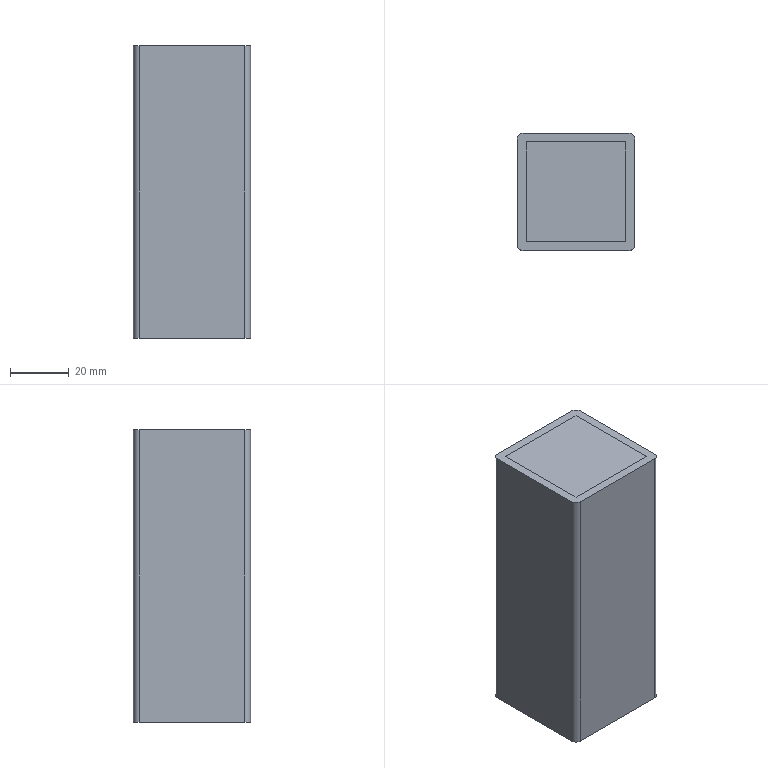Part | STEP file | X77-09105 | 2 solids | 20 faces | box 40 x 40 x 100 mm | volume 48681 mm3 | plane 16 | cylinder 4 | commonest cylinder face diameters 4 x4
STEP:
#1=CARTESIAN_POINT('',(0.,2.,100.));
#2=VERTEX_POINT('',#1);
#3=CARTESIAN_POINT('',(2.,0.,100.));
#4=VERTEX_POINT('',#3);
#5=CARTESIAN_POINT('',(2.,2.,100.));
#6=DIRECTION('',(0.,0.,1.));
#7=DIRECTION('',(1.,0.,0.));
#8=AXIS2_PLACEMENT_3D('',#5,#6,#7);
#9=CIRCLE('',#8,2.);
#10=EDGE_CURVE('',#2,#4,#9,.T.);
#11=ORIENTED_EDGE('',*,*,#10,.T.);
#12=CARTESIAN_POINT('',(38.,0.,100.));
#13=VERTEX_POINT('',#12);
#14=CARTESIAN_POINT('',(2.,0.,100.));
#15=DIRECTION('',(1.,0.,0.));
#16=VECTOR('',#15,1000.);
#17=LINE('',#14,#16);
#18=EDGE_CURVE('',#4,#13,#17,.T.);
#19=ORIENTED_EDGE('',*,*,#18,.T.);
#20=CARTESIAN_POINT('',(40.,2.,100.));
#21=VERTEX_POINT('',#20);
#22=CARTESIAN_POINT('',(38.,2.,100.));
#23=DIRECTION('',(0.,0.,1.));
#24=DIRECTION('',(1.,0.,0.));
#25=AXIS2_PLACEMENT_3D('',#22,#23,#24);
#26=CIRCLE('',#25,2.);
#27=EDGE_CURVE('',#13,#21,#26,.T.);
#28=ORIENTED_EDGE('',*,*,#27,.T.);
#29=CARTESIAN_POINT('',(40.,38.,100.));
#30=VERTEX_POINT('',#29);
#31=CARTESIAN_POINT('',(40.,2.,100.));
#32=DIRECTION('',(0.,1.,0.));
#33=VECTOR('',#32,1000.);
#34=LINE('',#31,#33);
#35=EDGE_CURVE('',#21,#30,#34,.T.);
#36=ORIENTED_EDGE('',*,*,#35,.T.);
#37=CARTESIAN_POINT('',(38.,40.,100.));
#38=VERTEX_POINT('',#37);
#39=CARTESIAN_POINT('',(38.,38.,100.));
#40=DIRECTION('',(0.,0.,1.));
#41=DIRECTION('',(1.,0.,0.));
#42=AXIS2_PLACEMENT_3D('',#39,#40,#41);
#43=CIRCLE('',#42,2.);
#44=EDGE_CURVE('',#30,#38,#43,.T.);
#45=ORIENTED_EDGE('',*,*,#44,.T.);
#46=CARTESIAN_POINT('',(2.,40.,100.));
#47=VERTEX_POINT('',#46);
#48=CARTESIAN_POINT('',(2.,40.,100.));
#49=DIRECTION('',(-1.,0.,0.));
#50=VECTOR('',#49,1000.);
#51=LINE('',#48,#50);
#52=EDGE_CURVE('',#38,#47,#51,.T.);
#53=ORIENTED_EDGE('',*,*,#52,.T.);
#54=CARTESIAN_POINT('',(0.,38.,100.));
#55=VERTEX_POINT('',#54);
#56=CARTESIAN_POINT('',(2.,38.,100.));
#57=DIRECTION('',(0.,0.,1.));
#58=DIRECTION('',(-1.,0.,0.));
#59=AXIS2_PLACEMENT_3D('',#56,#57,#58);
#60=CIRCLE('',#59,2.);
#61=EDGE_CURVE('',#47,#55,#60,.T.);
#62=ORIENTED_EDGE('',*,*,#61,.T.);
#63=CARTESIAN_POINT('',(0.,2.,100.));
#64=DIRECTION('',(0.,-1.,0.));
#65=VECTOR('',#64,1000.);
#66=LINE('',#63,#65);
#67=EDGE_CURVE('',#55,#2,#66,.T.);
#68=ORIENTED_EDGE('',*,*,#67,.T.);
#69=EDGE_LOOP('',(#11,#19,#28,#36,#45,#53,#62,#68));
#70=FACE_OUTER_BOUND('',#69,.T.);
#71=CARTESIAN_POINT('',(3.,3.,100.));
#72=VERTEX_POINT('',#71);
#73=CARTESIAN_POINT('',(37.,3.,100.));
#74=VERTEX_POINT('',#73);
#75=CARTESIAN_POINT('',(3.,3.,100.));
#76=DIRECTION('',(1.,0.,0.));
#77=VECTOR('',#76,1000.);
#78=LINE('',#75,#77);
#79=EDGE_CURVE('',#72,#74,#78,.T.);
#80=ORIENTED_EDGE('',*,*,#79,.F.);
#81=CARTESIAN_POINT('',(3.,37.,100.));
#82=VERTEX_POINT('',#81);
#83=CARTESIAN_POINT('',(3.,3.,100.));
#84=DIRECTION('',(0.,-1.,0.));
#85=VECTOR('',#84,1000.);
#86=LINE('',#83,#85);
#87=EDGE_CURVE('',#82,#72,#86,.T.);
#88=ORIENTED_EDGE('',*,*,#87,.F.);
#89=CARTESIAN_POINT('',(37.,37.,100.));
#90=VERTEX_POINT('',#89);
#91=CARTESIAN_POINT('',(3.,37.,100.));
#92=DIRECTION('',(-1.,0.,0.));
#93=VECTOR('',#92,1000.);
#94=LINE('',#91,#93);
#95=EDGE_CURVE('',#90,#82,#94,.T.);
#96=ORIENTED_EDGE('',*,*,#95,.F.);
#97=CARTESIAN_POINT('',(37.,3.,100.));
#98=DIRECTION('',(0.,1.,0.));
#99=VECTOR('',#98,1000.);
#100=LINE('',#97,#99);
#101=EDGE_CURVE('',#74,#90,#100,.T.);
#102=ORIENTED_EDGE('',*,*,#101,.F.);
#103=EDGE_LOOP('',(#80,#88,#96,#102));
#104=FACE_BOUND('',#103,.T.);
#105=CARTESIAN_POINT('',(2.,2.,100.));
#106=DIRECTION('',(0.,0.,1.));
#107=DIRECTION('',(1.,0.,0.));
#108=AXIS2_PLACEMENT_3D('',#105,#106,#107);
#109=PLANE('',#108);
#110=ADVANCED_FACE('',(#70,#104),#109,.T.);
#111=CARTESIAN_POINT('',(0.,2.,0.));
#112=VERTEX_POINT('',#111);
#113=CARTESIAN_POINT('',(2.,0.,0.));
#114=VERTEX_POINT('',#113);
#115=CARTESIAN_POINT('',(2.,2.,0.));
#116=DIRECTION('',(0.,0.,1.));
#117=DIRECTION('',(1.,0.,0.));
#118=AXIS2_PLACEMENT_3D('',#115,#116,#117);
#119=CIRCLE('',#118,2.);
#120=EDGE_CURVE('',#112,#114,#119,.T.);
#121=ORIENTED_EDGE('',*,*,#120,.F.);
#122=CARTESIAN_POINT('',(0.,38.,0.));
#123=VERTEX_POINT('',#122);
#124=CARTESIAN_POINT('',(0.,2.,0.));
#125=DIRECTION('',(0.,-1.,0.));
#126=VECTOR('',#125,1000.);
#127=LINE('',#124,#126);
#128=EDGE_CURVE('',#123,#112,#127,.T.);
#129=ORIENTED_EDGE('',*,*,#128,.F.);
#130=CARTESIAN_POINT('',(2.,40.,0.));
#131=VERTEX_POINT('',#130);
#132=CARTESIAN_POINT('',(2.,38.,0.));
#133=DIRECTION('',(0.,0.,1.));
#134=DIRECTION('',(-1.,0.,0.));
#135=AXIS2_PLACEMENT_3D('',#132,#133,#134);
#136=CIRCLE('',#135,2.);
#137=EDGE_CURVE('',#131,#123,#136,.T.);
#138=ORIENTED_EDGE('',*,*,#137,.F.);
#139=CARTESIAN_POINT('',(38.,40.,0.));
#140=VERTEX_POINT('',#139);
#141=CARTESIAN_POINT('',(2.,40.,0.));
#142=DIRECTION('',(-1.,0.,0.));
#143=VECTOR('',#142,1000.);
#144=LINE('',#141,#143);
#145=EDGE_CURVE('',#140,#131,#144,.T.);
#146=ORIENTED_EDGE('',*,*,#145,.F.);
#147=CARTESIAN_POINT('',(40.,38.,0.));
#148=VERTEX_POINT('',#147);
#149=CARTESIAN_POINT('',(38.,38.,0.));
#150=DIRECTION('',(0.,0.,1.));
#151=DIRECTION('',(1.,0.,0.));
#152=AXIS2_PLACEMENT_3D('',#149,#150,#151);
#153=CIRCLE('',#152,2.);
#154=EDGE_CURVE('',#148,#140,#153,.T.);
#155=ORIENTED_EDGE('',*,*,#154,.F.);
#156=CARTESIAN_POINT('',(40.,2.,0.));
#157=VERTEX_POINT('',#156);
#158=CARTESIAN_POINT('',(40.,2.,0.));
#159=DIRECTION('',(0.,1.,0.));
#160=VECTOR('',#159,1000.);
#161=LINE('',#158,#160);
#162=EDGE_CURVE('',#157,#148,#161,.T.);
#163=ORIENTED_EDGE('',*,*,#162,.F.);
#164=CARTESIAN_POINT('',(38.,0.,0.));
#165=VERTEX_POINT('',#164);
#166=CARTESIAN_POINT('',(38.,2.,0.));
#167=DIRECTION('',(0.,0.,1.));
#168=DIRECTION('',(1.,0.,0.));
#169=AXIS2_PLACEMENT_3D('',#166,#167,#168);
#170=CIRCLE('',#169,2.);
#171=EDGE_CURVE('',#165,#157,#170,.T.);
#172=ORIENTED_EDGE('',*,*,#171,.F.);
#173=CARTESIAN_POINT('',(2.,0.,0.));
#174=DIRECTION('',(1.,0.,0.));
#175=VECTOR('',#174,1000.);
#176=LINE('',#173,#175);
#177=EDGE_CURVE('',#114,#165,#176,.T.);
#178=ORIENTED_EDGE('',*,*,#177,.F.);
#179=EDGE_LOOP('',(#121,#129,#138,#146,#155,#163,#172,#178));
#180=FACE_OUTER_BOUND('',#179,.T.);
#181=CARTESIAN_POINT('',(3.,37.,0.));
#182=VERTEX_POINT('',#181);
#183=CARTESIAN_POINT('',(3.,3.,0.));
#184=VERTEX_POINT('',#183);
#185=CARTESIAN_POINT('',(3.,3.,0.));
#186=DIRECTION('',(0.,-1.,0.));
#187=VECTOR('',#186,1000.);
#188=LINE('',#185,#187);
#189=EDGE_CURVE('',#182,#184,#188,.T.);
#190=ORIENTED_EDGE('',*,*,#189,.T.);
#191=CARTESIAN_POINT('',(37.,3.,0.));
#192=VERTEX_POINT('',#191);
#193=CARTESIAN_POINT('',(3.,3.,0.));
#194=DIRECTION('',(1.,0.,0.));
#195=VECTOR('',#194,1000.);
#196=LINE('',#193,#195);
#197=EDGE_CURVE('',#184,#192,#196,.T.);
#198=ORIENTED_EDGE('',*,*,#197,.T.);
#199=CARTESIAN_POINT('',(37.,37.,0.));
#200=VERTEX_POINT('',#199);
#201=CARTESIAN_POINT('',(37.,3.,0.));
#202=DIRECTION('',(0.,1.,0.));
#203=VECTOR('',#202,1000.);
#204=LINE('',#201,#203);
#205=EDGE_CURVE('',#192,#200,#204,.T.);
#206=ORIENTED_EDGE('',*,*,#205,.T.);
#207=CARTESIAN_POINT('',(3.,37.,0.));
#208=DIRECTION('',(-1.,0.,0.));
#209=VECTOR('',#208,1000.);
#210=LINE('',#207,#209);
#211=EDGE_CURVE('',#200,#182,#210,.T.);
#212=ORIENTED_EDGE('',*,*,#211,.T.);
#213=EDGE_LOOP('',(#190,#198,#206,#212));
#214=FACE_BOUND('',#213,.T.);
#215=CARTESIAN_POINT('',(2.,2.,0.));
#216=DIRECTION('',(0.,0.,1.));
#217=DIRECTION('',(1.,0.,0.));
#218=AXIS2_PLACEMENT_3D('',#215,#216,#217);
#219=PLANE('',#218);
#220=ADVANCED_FACE('',(#180,#214),#219,.F.);
#221=ORIENTED_EDGE('',*,*,#120,.T.);
#222=CARTESIAN_POINT('',(2.,0.,100.));
#223=DIRECTION('',(0.,0.,-1.));
#224=VECTOR('',#223,1000.);
#225=LINE('',#222,#224);
#226=EDGE_CURVE('',#4,#114,#225,.T.);
#227=ORIENTED_EDGE('',*,*,#226,.F.);
#228=ORIENTED_EDGE('',*,*,#10,.F.);
#229=CARTESIAN_POINT('',(0.,2.,100.));
#230=DIRECTION('',(0.,0.,-1.));
#231=VECTOR('',#230,1000.);
#232=LINE('',#229,#231);
#233=EDGE_CURVE('',#2,#112,#232,.T.);
#234=ORIENTED_EDGE('',*,*,#233,.T.);
#235=EDGE_LOOP('',(#221,#227,#228,#234));
#236=FACE_OUTER_BOUND('',#235,.T.);
#237=CARTESIAN_POINT('',(2.,2.,100.));
#238=DIRECTION('',(0.,0.,-1.));
#239=DIRECTION('',(-1.,0.,0.));
#240=AXIS2_PLACEMENT_3D('',#237,#238,#239);
#241=CYLINDRICAL_SURFACE('',#240,2.);
#242=ADVANCED_FACE('',(#236),#241,.T.);
#243=ORIENTED_EDGE('',*,*,#177,.T.);
#244=CARTESIAN_POINT('',(38.,0.,100.));
#245=DIRECTION('',(0.,0.,-1.));
#246=VECTOR('',#245,1000.);
#247=LINE('',#244,#246);
#248=EDGE_CURVE('',#13,#165,#247,.T.);
#249=ORIENTED_EDGE('',*,*,#248,.F.);
#250=ORIENTED_EDGE('',*,*,#18,.F.);
#251=ORIENTED_EDGE('',*,*,#226,.T.);
#252=EDGE_LOOP('',(#243,#249,#250,#251));
#253=FACE_OUTER_BOUND('',#252,.T.);
#254=CARTESIAN_POINT('',(2.,0.,100.));
#255=DIRECTION('',(0.,1.,0.));
#256=DIRECTION('',(0.,0.,1.));
#257=AXIS2_PLACEMENT_3D('',#254,#255,#256);
#258=PLANE('',#257);
#259=ADVANCED_FACE('',(#253),#258,.F.);
#260=ORIENTED_EDGE('',*,*,#171,.T.);
#261=CARTESIAN_POINT('',(40.,2.,100.));
#262=DIRECTION('',(0.,0.,-1.));
#263=VECTOR('',#262,1000.);
#264=LINE('',#261,#263);
#265=EDGE_CURVE('',#21,#157,#264,.T.);
#266=ORIENTED_EDGE('',*,*,#265,.F.);
#267=ORIENTED_EDGE('',*,*,#27,.F.);
#268=ORIENTED_EDGE('',*,*,#248,.T.);
#269=EDGE_LOOP('',(#260,#266,#267,#268));
#270=FACE_OUTER_BOUND('',#269,.T.);
#271=CARTESIAN_POINT('',(38.,2.,100.));
#272=DIRECTION('',(0.,0.,-1.));
#273=DIRECTION('',(-1.,0.,0.));
#274=AXIS2_PLACEMENT_3D('',#271,#272,#273);
#275=CYLINDRICAL_SURFACE('',#274,2.);
#276=ADVANCED_FACE('',(#270),#275,.T.);
#277=ORIENTED_EDGE('',*,*,#162,.T.);
#278=CARTESIAN_POINT('',(40.,38.,100.));
#279=DIRECTION('',(0.,0.,-1.));
#280=VECTOR('',#279,1000.);
#281=LINE('',#278,#280);
#282=EDGE_CURVE('',#30,#148,#281,.T.);
#283=ORIENTED_EDGE('',*,*,#282,.F.);
#284=ORIENTED_EDGE('',*,*,#35,.F.);
#285=ORIENTED_EDGE('',*,*,#265,.T.);
#286=EDGE_LOOP('',(#277,#283,#284,#285));
#287=FACE_OUTER_BOUND('',#286,.T.);
#288=CARTESIAN_POINT('',(40.,2.,100.));
#289=DIRECTION('',(-1.,0.,0.));
#290=DIRECTION('',(0.,-1.,0.));
#291=AXIS2_PLACEMENT_3D('',#288,#289,#290);
#292=PLANE('',#291);
#293=ADVANCED_FACE('',(#287),#292,.F.);
#294=ORIENTED_EDGE('',*,*,#154,.T.);
#295=CARTESIAN_POINT('',(38.,40.,100.));
#296=DIRECTION('',(0.,0.,-1.));
#297=VECTOR('',#296,1000.);
#298=LINE('',#295,#297);
#299=EDGE_CURVE('',#38,#140,#298,.T.);
#300=ORIENTED_EDGE('',*,*,#299,.F.);
#301=ORIENTED_EDGE('',*,*,#44,.F.);
#302=ORIENTED_EDGE('',*,*,#282,.T.);
#303=EDGE_LOOP('',(#294,#300,#301,#302));
#304=FACE_OUTER_BOUND('',#303,.T.);
#305=CARTESIAN_POINT('',(38.,38.,100.));
#306=DIRECTION('',(0.,0.,-1.));
#307=DIRECTION('',(-1.,0.,0.));
#308=AXIS2_PLACEMENT_3D('',#305,#306,#307);
#309=CYLINDRICAL_SURFACE('',#308,2.);
#310=ADVANCED_FACE('',(#304),#309,.T.);
#311=ORIENTED_EDGE('',*,*,#145,.T.);
#312=CARTESIAN_POINT('',(2.,40.,100.));
#313=DIRECTION('',(0.,0.,-1.));
#314=VECTOR('',#313,1000.);
#315=LINE('',#312,#314);
#316=EDGE_CURVE('',#47,#131,#315,.T.);
#317=ORIENTED_EDGE('',*,*,#316,.F.);
#318=ORIENTED_EDGE('',*,*,#52,.F.);
#319=ORIENTED_EDGE('',*,*,#299,.T.);
#320=EDGE_LOOP('',(#311,#317,#318,#319));
#321=FACE_OUTER_BOUND('',#320,.T.);
#322=CARTESIAN_POINT('',(2.,40.,100.));
#323=DIRECTION('',(0.,-1.,0.));
#324=DIRECTION('',(0.,0.,-1.));
#325=AXIS2_PLACEMENT_3D('',#322,#323,#324);
#326=PLANE('',#325);
#327=ADVANCED_FACE('',(#321),#326,.F.);
#328=ORIENTED_EDGE('',*,*,#137,.T.);
#329=CARTESIAN_POINT('',(0.,38.,100.));
#330=DIRECTION('',(0.,0.,-1.));
#331=VECTOR('',#330,1000.);
#332=LINE('',#329,#331);
#333=EDGE_CURVE('',#55,#123,#332,.T.);
#334=ORIENTED_EDGE('',*,*,#333,.F.);
#335=ORIENTED_EDGE('',*,*,#61,.F.);
#336=ORIENTED_EDGE('',*,*,#316,.T.);
#337=EDGE_LOOP('',(#328,#334,#335,#336));
#338=FACE_OUTER_BOUND('',#337,.T.);
#339=CARTESIAN_POINT('',(2.,38.,100.));
#340=DIRECTION('',(0.,0.,-1.));
#341=DIRECTION('',(-1.,0.,0.));
#342=AXIS2_PLACEMENT_3D('',#339,#340,#341);
#343=CYLINDRICAL_SURFACE('',#342,2.);
#344=ADVANCED_FACE('',(#338),#343,.T.);
#345=ORIENTED_EDGE('',*,*,#128,.T.);
#346=ORIENTED_EDGE('',*,*,#233,.F.);
#347=ORIENTED_EDGE('',*,*,#67,.F.);
#348=ORIENTED_EDGE('',*,*,#333,.T.);
#349=EDGE_LOOP('',(#345,#346,#347,#348));
#350=FACE_OUTER_BOUND('',#349,.T.);
#351=CARTESIAN_POINT('',(0.,2.,100.));
#352=DIRECTION('',(1.,0.,0.));
#353=DIRECTION('',(0.,1.,0.));
#354=AXIS2_PLACEMENT_3D('',#351,#352,#353);
#355=PLANE('',#354);
#356=ADVANCED_FACE('',(#350),#355,.F.);
#357=ORIENTED_EDGE('',*,*,#189,.F.);
#358=CARTESIAN_POINT('',(3.,37.,100.));
#359=DIRECTION('',(0.,0.,-1.));
#360=VECTOR('',#359,1000.);
#361=LINE('',#358,#360);
#362=EDGE_CURVE('',#82,#182,#361,.T.);
#363=ORIENTED_EDGE('',*,*,#362,.F.);
#364=ORIENTED_EDGE('',*,*,#87,.T.);
#365=CARTESIAN_POINT('',(3.,3.,100.));
#366=DIRECTION('',(0.,0.,-1.));
#367=VECTOR('',#366,1000.);
#368=LINE('',#365,#367);
#369=EDGE_CURVE('',#72,#184,#368,.T.);
#370=ORIENTED_EDGE('',*,*,#369,.T.);
#371=EDGE_LOOP('',(#357,#363,#364,#370));
#372=FACE_OUTER_BOUND('',#371,.T.);
#373=CARTESIAN_POINT('',(3.,3.,100.));
#374=DIRECTION('',(1.,0.,0.));
#375=DIRECTION('',(0.,0.,-1.));
#376=AXIS2_PLACEMENT_3D('',#373,#374,#375);
#377=PLANE('',#376);
#378=ADVANCED_FACE('',(#372),#377,.T.);
#379=ORIENTED_EDGE('',*,*,#197,.F.);
#380=ORIENTED_EDGE('',*,*,#369,.F.);
#381=ORIENTED_EDGE('',*,*,#79,.T.);
#382=CARTESIAN_POINT('',(37.,3.,100.));
#383=DIRECTION('',(0.,0.,-1.));
#384=VECTOR('',#383,1000.);
#385=LINE('',#382,#384);
#386=EDGE_CURVE('',#74,#192,#385,.T.);
#387=ORIENTED_EDGE('',*,*,#386,.T.);
#388=EDGE_LOOP('',(#379,#380,#381,#387));
#389=FACE_OUTER_BOUND('',#388,.T.);
#390=CARTESIAN_POINT('',(3.,3.,100.));
#391=DIRECTION('',(0.,1.,0.));
#392=DIRECTION('',(0.,0.,1.));
#393=AXIS2_PLACEMENT_3D('',#390,#391,#392);
#394=PLANE('',#393);
#395=ADVANCED_FACE('',(#389),#394,.T.);
#396=ORIENTED_EDGE('',*,*,#205,.F.);
#397=ORIENTED_EDGE('',*,*,#386,.F.);
#398=ORIENTED_EDGE('',*,*,#101,.T.);
#399=CARTESIAN_POINT('',(37.,37.,100.));
#400=DIRECTION('',(0.,0.,-1.));
#401=VECTOR('',#400,1000.);
#402=LINE('',#399,#401);
#403=EDGE_CURVE('',#90,#200,#402,.T.);
#404=ORIENTED_EDGE('',*,*,#403,.T.);
#405=EDGE_LOOP('',(#396,#397,#398,#404));
#406=FACE_OUTER_BOUND('',#405,.T.);
#407=CARTESIAN_POINT('',(37.,3.,100.));
#408=DIRECTION('',(-1.,0.,0.));
#409=DIRECTION('',(0.,0.,1.));
#410=AXIS2_PLACEMENT_3D('',#407,#408,#409);
#411=PLANE('',#410);
#412=ADVANCED_FACE('',(#406),#411,.T.);
#413=ORIENTED_EDGE('',*,*,#211,.F.);
#414=ORIENTED_EDGE('',*,*,#403,.F.);
#415=ORIENTED_EDGE('',*,*,#95,.T.);
#416=ORIENTED_EDGE('',*,*,#362,.T.);
#417=EDGE_LOOP('',(#413,#414,#415,#416));
#418=FACE_OUTER_BOUND('',#417,.T.);
#419=CARTESIAN_POINT('',(3.,37.,100.));
#420=DIRECTION('',(0.,-1.,0.));
#421=DIRECTION('',(0.,0.,-1.));
#422=AXIS2_PLACEMENT_3D('',#419,#420,#421);
#423=PLANE('',#422);
#424=ADVANCED_FACE('',(#418),#423,.T.);
#425=CLOSED_SHELL('',(#110,#220,#242,#259,#276,#293,#310,#327,#344,#356,#378,#395,#412,#424));
#426=MANIFOLD_SOLID_BREP('',#425);
#427=CARTESIAN_POINT('',(3.,37.,100.));
#428=VERTEX_POINT('',#427);
#429=CARTESIAN_POINT('',(3.,3.,100.));
#430=VERTEX_POINT('',#429);
#431=CARTESIAN_POINT('',(3.,37.,100.));
#432=DIRECTION('',(0.,-1.,0.));
#433=VECTOR('',#432,1000.);
#434=LINE('',#431,#433);
#435=EDGE_CURVE('',#428,#430,#434,.T.);
#436=ORIENTED_EDGE('',*,*,#435,.F.);
#437=CARTESIAN_POINT('',(3.,37.,96.));
#438=VERTEX_POINT('',#437);
#439=CARTESIAN_POINT('',(3.,37.,96.));
#440=DIRECTION('',(0.,0.,1.));
#441=VECTOR('',#440,1000.);
#442=LINE('',#439,#441);
#443=EDGE_CURVE('',#438,#428,#442,.T.);
#444=ORIENTED_EDGE('',*,*,#443,.F.);
#445=CARTESIAN_POINT('',(3.,3.,96.));
#446=VERTEX_POINT('',#445);
#447=CARTESIAN_POINT('',(3.,37.,96.));
#448=DIRECTION('',(0.,-1.,0.));
#449=VECTOR('',#448,1000.);
#450=LINE('',#447,#449);
#451=EDGE_CURVE('',#438,#446,#450,.T.);
#452=ORIENTED_EDGE('',*,*,#451,.T.);
#453=CARTESIAN_POINT('',(3.,3.,96.));
#454=DIRECTION('',(0.,0.,1.));
#455=VECTOR('',#454,1000.);
#456=LINE('',#453,#455);
#457=EDGE_CURVE('',#446,#430,#456,.T.);
#458=ORIENTED_EDGE('',*,*,#457,.T.);
#459=EDGE_LOOP('',(#436,#444,#452,#458));
#460=FACE_OUTER_BOUND('',#459,.T.);
#461=CARTESIAN_POINT('',(3.,37.,96.));
#462=DIRECTION('',(-1.,0.,0.));
#463=DIRECTION('',(0.,0.,1.));
#464=AXIS2_PLACEMENT_3D('',#461,#462,#463);
#465=PLANE('',#464);
#466=ADVANCED_FACE('',(#460),#465,.T.);
#467=CARTESIAN_POINT('',(37.,37.,100.));
#468=VERTEX_POINT('',#467);
#469=CARTESIAN_POINT('',(3.,37.,100.));
#470=DIRECTION('',(-1.,0.,0.));
#471=VECTOR('',#470,1000.);
#472=LINE('',#469,#471);
#473=EDGE_CURVE('',#468,#428,#472,.T.);
#474=ORIENTED_EDGE('',*,*,#473,.F.);
#475=CARTESIAN_POINT('',(37.,37.,96.));
#476=VERTEX_POINT('',#475);
#477=CARTESIAN_POINT('',(37.,37.,96.));
#478=DIRECTION('',(0.,0.,1.));
#479=VECTOR('',#478,1000.);
#480=LINE('',#477,#479);
#481=EDGE_CURVE('',#476,#468,#480,.T.);
#482=ORIENTED_EDGE('',*,*,#481,.F.);
#483=CARTESIAN_POINT('',(3.,37.,96.));
#484=DIRECTION('',(-1.,0.,0.));
#485=VECTOR('',#484,1000.);
#486=LINE('',#483,#485);
#487=EDGE_CURVE('',#476,#438,#486,.T.);
#488=ORIENTED_EDGE('',*,*,#487,.T.);
#489=ORIENTED_EDGE('',*,*,#443,.T.);
#490=EDGE_LOOP('',(#474,#482,#488,#489));
#491=FACE_OUTER_BOUND('',#490,.T.);
#492=CARTESIAN_POINT('',(3.,37.,96.));
#493=DIRECTION('',(0.,1.,0.));
#494=DIRECTION('',(0.,0.,1.));
#495=AXIS2_PLACEMENT_3D('',#492,#493,#494);
#496=PLANE('',#495);
#497=ADVANCED_FACE('',(#491),#496,.T.);
#498=CARTESIAN_POINT('',(37.,3.,100.));
#499=VERTEX_POINT('',#498);
#500=CARTESIAN_POINT('',(37.,37.,100.));
#501=DIRECTION('',(0.,1.,0.));
#502=VECTOR('',#501,1000.);
#503=LINE('',#500,#502);
#504=EDGE_CURVE('',#499,#468,#503,.T.);
#505=ORIENTED_EDGE('',*,*,#504,.F.);
#506=CARTESIAN_POINT('',(37.,3.,96.));
#507=VERTEX_POINT('',#506);
#508=CARTESIAN_POINT('',(37.,3.,96.));
#509=DIRECTION('',(0.,0.,1.));
#510=VECTOR('',#509,1000.);
#511=LINE('',#508,#510);
#512=EDGE_CURVE('',#507,#499,#511,.T.);
#513=ORIENTED_EDGE('',*,*,#512,.F.);
#514=CARTESIAN_POINT('',(37.,37.,96.));
#515=DIRECTION('',(0.,1.,0.));
#516=VECTOR('',#515,1000.);
#517=LINE('',#514,#516);
#518=EDGE_CURVE('',#507,#476,#517,.T.);
#519=ORIENTED_EDGE('',*,*,#518,.T.);
#520=ORIENTED_EDGE('',*,*,#481,.T.);
#521=EDGE_LOOP('',(#505,#513,#519,#520));
#522=FACE_OUTER_BOUND('',#521,.T.);
#523=CARTESIAN_POINT('',(37.,37.,96.));
#524=DIRECTION('',(1.,0.,0.));
#525=DIRECTION('',(0.,0.,-1.));
#526=AXIS2_PLACEMENT_3D('',#523,#524,#525);
#527=PLANE('',#526);
#528=ADVANCED_FACE('',(#522),#527,.T.);
#529=CARTESIAN_POINT('',(3.,3.,100.));
#530=DIRECTION('',(1.,0.,0.));
#531=VECTOR('',#530,1000.);
#532=LINE('',#529,#531);
#533=EDGE_CURVE('',#430,#499,#532,.T.);
#534=ORIENTED_EDGE('',*,*,#533,.F.);
#535=ORIENTED_EDGE('',*,*,#457,.F.);
#536=CARTESIAN_POINT('',(3.,3.,96.));
#537=DIRECTION('',(1.,0.,0.));
#538=VECTOR('',#537,1000.);
#539=LINE('',#536,#538);
#540=EDGE_CURVE('',#446,#507,#539,.T.);
#541=ORIENTED_EDGE('',*,*,#540,.T.);
#542=ORIENTED_EDGE('',*,*,#512,.T.);
#543=EDGE_LOOP('',(#534,#535,#541,#542));
#544=FACE_OUTER_BOUND('',#543,.T.);
#545=CARTESIAN_POINT('',(3.,3.,96.));
#546=DIRECTION('',(0.,-1.,0.));
#547=DIRECTION('',(0.,0.,-1.));
#548=AXIS2_PLACEMENT_3D('',#545,#546,#547);
#549=PLANE('',#548);
#550=ADVANCED_FACE('',(#544),#549,.T.);
#551=ORIENTED_EDGE('',*,*,#451,.F.);
#552=ORIENTED_EDGE('',*,*,#487,.F.);
#553=ORIENTED_EDGE('',*,*,#518,.F.);
#554=ORIENTED_EDGE('',*,*,#540,.F.);
#555=EDGE_LOOP('',(#551,#552,#553,#554));
#556=FACE_OUTER_BOUND('',#555,.T.);
#557=CARTESIAN_POINT('',(3.,3.,96.));
#558=DIRECTION('',(0.,0.,1.));
#559=DIRECTION('',(1.,0.,0.));
#560=AXIS2_PLACEMENT_3D('',#557,#558,#559);
#561=PLANE('',#560);
#562=ADVANCED_FACE('',(#556),#561,.F.);
#563=ORIENTED_EDGE('',*,*,#435,.T.);
#564=ORIENTED_EDGE('',*,*,#533,.T.);
#565=ORIENTED_EDGE('',*,*,#504,.T.);
#566=ORIENTED_EDGE('',*,*,#473,.T.);
#567=EDGE_LOOP('',(#563,#564,#565,#566));
#568=FACE_OUTER_BOUND('',#567,.T.);
#569=CARTESIAN_POINT('',(3.,3.,100.));
#570=DIRECTION('',(0.,0.,1.));
#571=DIRECTION('',(1.,0.,0.));
#572=AXIS2_PLACEMENT_3D('',#569,#570,#571);
#573=PLANE('',#572);
#574=ADVANCED_FACE('',(#568),#573,.T.);
#575=CLOSED_SHELL('',(#466,#497,#528,#550,#562,#574));
#576=MANIFOLD_SOLID_BREP('',#575);
#577=CARTESIAN_POINT('',(0.,0.,0.));
#578=DIRECTION('',(0.,0.,1.));
#579=DIRECTION('',(1.,0.,0.));
#580=AXIS2_PLACEMENT_3D('',#577,#578,#579);
#581=(LENGTH_UNIT()NAMED_UNIT(*)SI_UNIT(.MILLI.,.METRE.));
#582=UNCERTAINTY_MEASURE_WITH_UNIT(LENGTH_MEASURE(0.00001),#581,'','');
#583=(NAMED_UNIT(*)PLANE_ANGLE_UNIT()SI_UNIT($,.RADIAN.));
#584=(NAMED_UNIT(*)SI_UNIT($,.STERADIAN.)SOLID_ANGLE_UNIT());
#585=(GEOMETRIC_REPRESENTATION_CONTEXT(3)GLOBAL_UNCERTAINTY_ASSIGNED_CONTEXT((#582))GLOBAL_UNIT_ASSIGNED_CONTEXT((#581,#583,#584))REPRESENTATION_CONTEXT('',''));
#586=ADVANCED_BREP_SHAPE_REPRESENTATION('',(#426,#576,#580),#585);